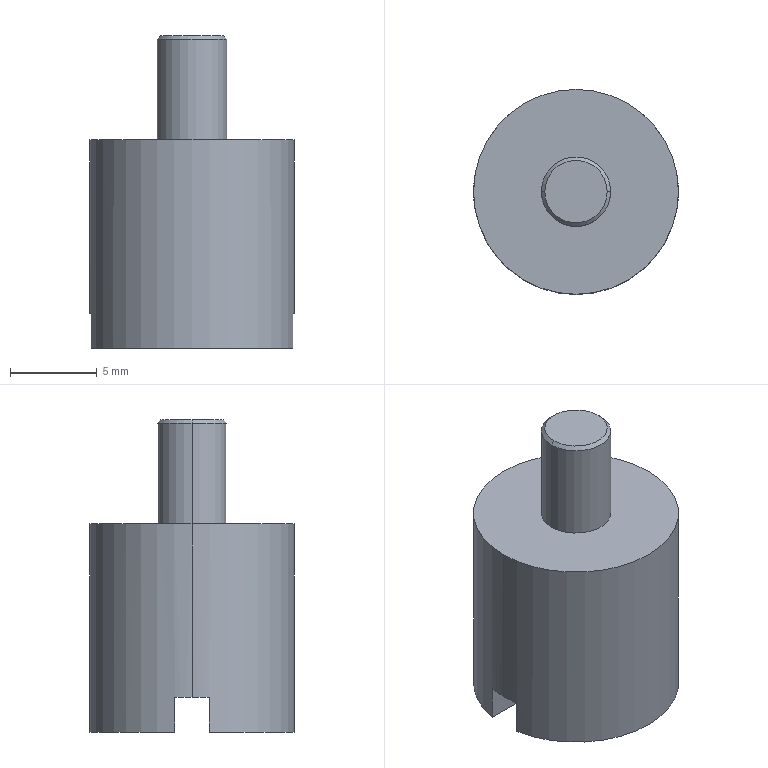Part | NX | features BREP 1 | 1 solid | 13 faces | box 11.8 x 11.8 x 18 mm | volume 1340 mm3 | plane 7 | cylinder 4 | cone 2 | commonest cylinder face diameters 4 x2 11.8 x2
STEP:
#1=CARTESIAN_POINT('',(-5.815,1.,2.));
#2=VERTEX_POINT('',#1);
#3=CARTESIAN_POINT('',(5.815,1.,2.));
#4=VERTEX_POINT('',#3);
#5=CARTESIAN_POINT('',(5.9,1.,2.));
#6=DIRECTION('',(1.,0.,0.));
#7=VECTOR('',#6,1000.);
#8=LINE('',#5,#7);
#9=EDGE_CURVE('',#2,#4,#8,.T.);
#10=ORIENTED_EDGE('',*,*,#9,.F.);
#11=CARTESIAN_POINT('',(-5.815,1.,0.));
#12=VERTEX_POINT('',#11);
#13=CARTESIAN_POINT('',(-5.815,1.,12.));
#14=DIRECTION('',(0.,0.,1.));
#15=VECTOR('',#14,1000.);
#16=LINE('',#13,#15);
#17=EDGE_CURVE('',#12,#2,#16,.T.);
#18=ORIENTED_EDGE('',*,*,#17,.F.);
#19=CARTESIAN_POINT('',(5.815,1.,0.));
#20=VERTEX_POINT('',#19);
#21=CARTESIAN_POINT('',(0.,1.,0.));
#22=DIRECTION('',(-1.,0.,0.));
#23=VECTOR('',#22,1000.);
#24=LINE('',#21,#23);
#25=EDGE_CURVE('',#20,#12,#24,.T.);
#26=ORIENTED_EDGE('',*,*,#25,.F.);
#27=CARTESIAN_POINT('',(5.815,1.,12.));
#28=DIRECTION('',(0.,0.,-1.));
#29=VECTOR('',#28,1000.);
#30=LINE('',#27,#29);
#31=EDGE_CURVE('',#4,#20,#30,.T.);
#32=ORIENTED_EDGE('',*,*,#31,.F.);
#33=EDGE_LOOP('',(#10,#18,#26,#32));
#34=FACE_BOUND('',#33,.T.);
#35=CARTESIAN_POINT('',(5.9,1.,2.));
#36=DIRECTION('',(0.,1.,0.));
#37=DIRECTION('',(0.,0.,1.));
#38=AXIS2_PLACEMENT_3D('',#35,#36,#37);
#39=PLANE('',#38);
#40=ADVANCED_FACE('',(#34),#39,.F.);
#41=CARTESIAN_POINT('',(5.815,-1.,2.));
#42=VERTEX_POINT('',#41);
#43=CARTESIAN_POINT('',(-5.815,-1.,2.));
#44=VERTEX_POINT('',#43);
#45=CARTESIAN_POINT('',(5.9,-1.,2.));
#46=DIRECTION('',(-1.,0.,0.));
#47=VECTOR('',#46,1000.);
#48=LINE('',#45,#47);
#49=EDGE_CURVE('',#42,#44,#48,.T.);
#50=ORIENTED_EDGE('',*,*,#49,.F.);
#51=CARTESIAN_POINT('',(5.815,-1.,0.));
#52=VERTEX_POINT('',#51);
#53=CARTESIAN_POINT('',(5.815,-1.,12.));
#54=DIRECTION('',(0.,0.,1.));
#55=VECTOR('',#54,1000.);
#56=LINE('',#53,#55);
#57=EDGE_CURVE('',#52,#42,#56,.T.);
#58=ORIENTED_EDGE('',*,*,#57,.F.);
#59=CARTESIAN_POINT('',(-5.815,-1.,0.));
#60=VERTEX_POINT('',#59);
#61=CARTESIAN_POINT('',(0.,-1.,0.));
#62=DIRECTION('',(1.,0.,0.));
#63=VECTOR('',#62,1000.);
#64=LINE('',#61,#63);
#65=EDGE_CURVE('',#60,#52,#64,.T.);
#66=ORIENTED_EDGE('',*,*,#65,.F.);
#67=CARTESIAN_POINT('',(-5.815,-1.,12.));
#68=DIRECTION('',(0.,0.,-1.));
#69=VECTOR('',#68,1000.);
#70=LINE('',#67,#69);
#71=EDGE_CURVE('',#44,#60,#70,.T.);
#72=ORIENTED_EDGE('',*,*,#71,.F.);
#73=EDGE_LOOP('',(#50,#58,#66,#72));
#74=FACE_BOUND('',#73,.T.);
#75=CARTESIAN_POINT('',(5.9,-1.,2.));
#76=DIRECTION('',(0.,-1.,0.));
#77=DIRECTION('',(0.,0.,-1.));
#78=AXIS2_PLACEMENT_3D('',#75,#76,#77);
#79=PLANE('',#78);
#80=ADVANCED_FACE('',(#74),#79,.F.);
#81=ORIENTED_EDGE('',*,*,#9,.T.);
#82=CARTESIAN_POINT('',(5.9,0.,2.));
#83=VERTEX_POINT('',#82);
#84=CARTESIAN_POINT('',(0.,0.,2.));
#85=DIRECTION('',(0.,0.,1.));
#86=DIRECTION('',(1.,0.,0.));
#87=AXIS2_PLACEMENT_3D('',#84,#85,#86);
#88=CIRCLE('',#87,5.9);
#89=EDGE_CURVE('',#83,#4,#88,.T.);
#90=ORIENTED_EDGE('',*,*,#89,.F.);
#91=CARTESIAN_POINT('',(0.,0.,2.));
#92=DIRECTION('',(0.,0.,1.));
#93=DIRECTION('',(1.,0.,0.));
#94=AXIS2_PLACEMENT_3D('',#91,#92,#93);
#95=CIRCLE('',#94,5.9);
#96=EDGE_CURVE('',#42,#83,#95,.T.);
#97=ORIENTED_EDGE('',*,*,#96,.F.);
#98=ORIENTED_EDGE('',*,*,#49,.T.);
#99=CARTESIAN_POINT('',(-5.9,0.,2.));
#100=VERTEX_POINT('',#99);
#101=CARTESIAN_POINT('',(0.,0.,2.));
#102=DIRECTION('',(0.,0.,1.));
#103=DIRECTION('',(1.,0.,0.));
#104=AXIS2_PLACEMENT_3D('',#101,#102,#103);
#105=CIRCLE('',#104,5.9);
#106=EDGE_CURVE('',#100,#44,#105,.T.);
#107=ORIENTED_EDGE('',*,*,#106,.F.);
#108=CARTESIAN_POINT('',(0.,0.,2.));
#109=DIRECTION('',(0.,0.,1.));
#110=DIRECTION('',(1.,0.,0.));
#111=AXIS2_PLACEMENT_3D('',#108,#109,#110);
#112=CIRCLE('',#111,5.9);
#113=EDGE_CURVE('',#2,#100,#112,.T.);
#114=ORIENTED_EDGE('',*,*,#113,.F.);
#115=EDGE_LOOP('',(#81,#90,#97,#98,#107,#114));
#116=FACE_BOUND('',#115,.T.);
#117=CARTESIAN_POINT('',(0.,0.,2.));
#118=DIRECTION('',(0.,0.,1.));
#119=DIRECTION('',(1.,0.,0.));
#120=AXIS2_PLACEMENT_3D('',#117,#118,#119);
#121=PLANE('',#120);
#122=ADVANCED_FACE('',(#116),#121,.F.);
#123=CARTESIAN_POINT('',(1.8,0.,18.));
#124=VERTEX_POINT('',#123);
#125=CARTESIAN_POINT('',(2.,0.,17.8));
#126=VERTEX_POINT('',#125);
#127=CARTESIAN_POINT('',(1.8,0.,18.));
#128=DIRECTION('',(0.7071,0.,-0.7071));
#129=VECTOR('',#128,1000.);
#130=LINE('',#127,#129);
#131=EDGE_CURVE('',#124,#126,#130,.T.);
#132=ORIENTED_EDGE('',*,*,#131,.F.);
#133=CARTESIAN_POINT('',(-1.8,0.,18.));
#134=VERTEX_POINT('',#133);
#135=CARTESIAN_POINT('',(0.,0.,18.));
#136=DIRECTION('',(0.,0.,1.));
#137=DIRECTION('',(1.,0.,0.));
#138=AXIS2_PLACEMENT_3D('',#135,#136,#137);
#139=CIRCLE('',#138,1.8);
#140=EDGE_CURVE('',#134,#124,#139,.T.);
#141=ORIENTED_EDGE('',*,*,#140,.F.);
#142=CARTESIAN_POINT('',(-2.,0.,17.8));
#143=VERTEX_POINT('',#142);
#144=CARTESIAN_POINT('',(-1.8,0.,18.));
#145=DIRECTION('',(-0.7071,0.,-0.7071));
#146=VECTOR('',#145,1000.);
#147=LINE('',#144,#146);
#148=EDGE_CURVE('',#134,#143,#147,.T.);
#149=ORIENTED_EDGE('',*,*,#148,.T.);
#150=CARTESIAN_POINT('',(0.,0.,17.8));
#151=DIRECTION('',(0.,0.,-1.));
#152=DIRECTION('',(1.,0.,0.));
#153=AXIS2_PLACEMENT_3D('',#150,#151,#152);
#154=CIRCLE('',#153,2.);
#155=EDGE_CURVE('',#126,#143,#154,.T.);
#156=ORIENTED_EDGE('',*,*,#155,.F.);
#157=EDGE_LOOP('',(#132,#141,#149,#156));
#158=FACE_BOUND('',#157,.T.);
#159=CARTESIAN_POINT('',(0.,0.,18.));
#160=DIRECTION('',(0.,0.,-1.));
#161=DIRECTION('',(-1.,0.,0.));
#162=AXIS2_PLACEMENT_3D('',#159,#160,#161);
#163=CONICAL_SURFACE('',#162,1.8,0.7854);
#164=ADVANCED_FACE('',(#158),#163,.T.);
#165=ORIENTED_EDGE('',*,*,#140,.T.);
#166=CARTESIAN_POINT('',(0.,0.,18.));
#167=DIRECTION('',(0.,0.,1.));
#168=DIRECTION('',(1.,0.,0.));
#169=AXIS2_PLACEMENT_3D('',#166,#167,#168);
#170=CIRCLE('',#169,1.8);
#171=EDGE_CURVE('',#124,#134,#170,.T.);
#172=ORIENTED_EDGE('',*,*,#171,.T.);
#173=EDGE_LOOP('',(#165,#172));
#174=FACE_BOUND('',#173,.T.);
#175=CARTESIAN_POINT('',(0.,0.,18.));
#176=DIRECTION('',(0.,0.,1.));
#177=DIRECTION('',(1.,0.,0.));
#178=AXIS2_PLACEMENT_3D('',#175,#176,#177);
#179=PLANE('',#178);
#180=ADVANCED_FACE('',(#174),#179,.T.);
#181=CARTESIAN_POINT('',(2.,0.,12.));
#182=VERTEX_POINT('',#181);
#183=CARTESIAN_POINT('',(2.,0.,18.));
#184=DIRECTION('',(0.,0.,-1.));
#185=VECTOR('',#184,1000.);
#186=LINE('',#183,#185);
#187=EDGE_CURVE('',#126,#182,#186,.T.);
#188=ORIENTED_EDGE('',*,*,#187,.F.);
#189=ORIENTED_EDGE('',*,*,#155,.T.);
#190=CARTESIAN_POINT('',(-2.,0.,12.));
#191=VERTEX_POINT('',#190);
#192=CARTESIAN_POINT('',(-2.,0.,18.));
#193=DIRECTION('',(0.,0.,-1.));
#194=VECTOR('',#193,1000.);
#195=LINE('',#192,#194);
#196=EDGE_CURVE('',#143,#191,#195,.T.);
#197=ORIENTED_EDGE('',*,*,#196,.T.);
#198=CARTESIAN_POINT('',(0.,0.,12.));
#199=DIRECTION('',(0.,0.,1.));
#200=DIRECTION('',(1.,0.,0.));
#201=AXIS2_PLACEMENT_3D('',#198,#199,#200);
#202=CIRCLE('',#201,2.);
#203=EDGE_CURVE('',#191,#182,#202,.T.);
#204=ORIENTED_EDGE('',*,*,#203,.T.);
#205=EDGE_LOOP('',(#188,#189,#197,#204));
#206=FACE_BOUND('',#205,.T.);
#207=CARTESIAN_POINT('',(0.,0.,18.));
#208=DIRECTION('',(0.,0.,-1.));
#209=DIRECTION('',(-1.,0.,0.));
#210=AXIS2_PLACEMENT_3D('',#207,#208,#209);
#211=CYLINDRICAL_SURFACE('',#210,2.);
#212=ADVANCED_FACE('',(#206),#211,.T.);
#213=CARTESIAN_POINT('',(0.,0.,0.));
#214=DIRECTION('',(0.,0.,1.));
#215=DIRECTION('',(1.,0.,0.));
#216=AXIS2_PLACEMENT_3D('',#213,#214,#215);
#217=CIRCLE('',#216,5.9);
#218=EDGE_CURVE('',#20,#12,#217,.T.);
#219=ORIENTED_EDGE('',*,*,#218,.F.);
#220=ORIENTED_EDGE('',*,*,#25,.T.);
#221=EDGE_LOOP('',(#219,#220));
#222=FACE_BOUND('',#221,.T.);
#223=CARTESIAN_POINT('',(0.,0.,0.));
#224=DIRECTION('',(0.,0.,1.));
#225=DIRECTION('',(1.,0.,0.));
#226=AXIS2_PLACEMENT_3D('',#223,#224,#225);
#227=PLANE('',#226);
#228=ADVANCED_FACE('',(#222),#227,.F.);
#229=CARTESIAN_POINT('',(-5.9,0.,12.));
#230=VERTEX_POINT('',#229);
#231=CARTESIAN_POINT('',(5.9,0.,12.));
#232=VERTEX_POINT('',#231);
#233=CARTESIAN_POINT('',(0.,0.,12.));
#234=DIRECTION('',(0.,0.,1.));
#235=DIRECTION('',(1.,0.,0.));
#236=AXIS2_PLACEMENT_3D('',#233,#234,#235);
#237=CIRCLE('',#236,5.9);
#238=EDGE_CURVE('',#230,#232,#237,.T.);
#239=ORIENTED_EDGE('',*,*,#238,.T.);
#240=CARTESIAN_POINT('',(0.,0.,12.));
#241=DIRECTION('',(0.,0.,1.));
#242=DIRECTION('',(1.,0.,0.));
#243=AXIS2_PLACEMENT_3D('',#240,#241,#242);
#244=CIRCLE('',#243,5.9);
#245=EDGE_CURVE('',#232,#230,#244,.T.);
#246=ORIENTED_EDGE('',*,*,#245,.T.);
#247=EDGE_LOOP('',(#239,#246));
#248=FACE_BOUND('',#247,.T.);
#249=ORIENTED_EDGE('',*,*,#203,.F.);
#250=CARTESIAN_POINT('',(0.,0.,12.));
#251=DIRECTION('',(0.,0.,1.));
#252=DIRECTION('',(1.,0.,0.));
#253=AXIS2_PLACEMENT_3D('',#250,#251,#252);
#254=CIRCLE('',#253,2.);
#255=EDGE_CURVE('',#182,#191,#254,.T.);
#256=ORIENTED_EDGE('',*,*,#255,.F.);
#257=EDGE_LOOP('',(#249,#256));
#258=FACE_BOUND('',#257,.T.);
#259=CARTESIAN_POINT('',(0.,0.,12.));
#260=DIRECTION('',(0.,0.,1.));
#261=DIRECTION('',(1.,0.,0.));
#262=AXIS2_PLACEMENT_3D('',#259,#260,#261);
#263=PLANE('',#262);
#264=ADVANCED_FACE('',(#248,#258),#263,.T.);
#265=CARTESIAN_POINT('',(5.9,0.,12.));
#266=DIRECTION('',(0.,0.,-1.));
#267=VECTOR('',#266,1000.);
#268=LINE('',#265,#267);
#269=EDGE_CURVE('',#232,#83,#268,.T.);
#270=ORIENTED_EDGE('',*,*,#269,.F.);
#271=ORIENTED_EDGE('',*,*,#238,.F.);
#272=CARTESIAN_POINT('',(-5.9,0.,12.));
#273=DIRECTION('',(0.,0.,-1.));
#274=VECTOR('',#273,1000.);
#275=LINE('',#272,#274);
#276=EDGE_CURVE('',#230,#100,#275,.T.);
#277=ORIENTED_EDGE('',*,*,#276,.T.);
#278=ORIENTED_EDGE('',*,*,#106,.T.);
#279=ORIENTED_EDGE('',*,*,#71,.T.);
#280=CARTESIAN_POINT('',(0.,0.,0.));
#281=DIRECTION('',(0.,0.,1.));
#282=DIRECTION('',(1.,0.,0.));
#283=AXIS2_PLACEMENT_3D('',#280,#281,#282);
#284=CIRCLE('',#283,5.9);
#285=EDGE_CURVE('',#60,#52,#284,.T.);
#286=ORIENTED_EDGE('',*,*,#285,.T.);
#287=ORIENTED_EDGE('',*,*,#57,.T.);
#288=ORIENTED_EDGE('',*,*,#96,.T.);
#289=EDGE_LOOP('',(#270,#271,#277,#278,#279,#286,#287,#288));
#290=FACE_BOUND('',#289,.T.);
#291=CARTESIAN_POINT('',(0.,0.,12.));
#292=DIRECTION('',(0.,0.,-1.));
#293=DIRECTION('',(-1.,0.,0.));
#294=AXIS2_PLACEMENT_3D('',#291,#292,#293);
#295=CYLINDRICAL_SURFACE('',#294,5.9);
#296=ADVANCED_FACE('',(#290),#295,.T.);
#297=ORIENTED_EDGE('',*,*,#285,.F.);
#298=ORIENTED_EDGE('',*,*,#65,.T.);
#299=EDGE_LOOP('',(#297,#298));
#300=FACE_BOUND('',#299,.T.);
#301=CARTESIAN_POINT('',(0.,0.,0.));
#302=DIRECTION('',(0.,0.,1.));
#303=DIRECTION('',(1.,0.,0.));
#304=AXIS2_PLACEMENT_3D('',#301,#302,#303);
#305=PLANE('',#304);
#306=ADVANCED_FACE('',(#300),#305,.F.);
#307=ORIENTED_EDGE('',*,*,#245,.F.);
#308=ORIENTED_EDGE('',*,*,#269,.T.);
#309=ORIENTED_EDGE('',*,*,#89,.T.);
#310=ORIENTED_EDGE('',*,*,#31,.T.);
#311=ORIENTED_EDGE('',*,*,#218,.T.);
#312=ORIENTED_EDGE('',*,*,#17,.T.);
#313=ORIENTED_EDGE('',*,*,#113,.T.);
#314=ORIENTED_EDGE('',*,*,#276,.F.);
#315=EDGE_LOOP('',(#307,#308,#309,#310,#311,#312,#313,#314));
#316=FACE_BOUND('',#315,.T.);
#317=CARTESIAN_POINT('',(0.,0.,12.));
#318=DIRECTION('',(0.,0.,-1.));
#319=DIRECTION('',(-1.,0.,0.));
#320=AXIS2_PLACEMENT_3D('',#317,#318,#319);
#321=CYLINDRICAL_SURFACE('',#320,5.9);
#322=ADVANCED_FACE('',(#316),#321,.T.);
#323=CARTESIAN_POINT('',(0.,0.,17.8));
#324=DIRECTION('',(0.,0.,-1.));
#325=DIRECTION('',(1.,0.,0.));
#326=AXIS2_PLACEMENT_3D('',#323,#324,#325);
#327=CIRCLE('',#326,2.);
#328=EDGE_CURVE('',#143,#126,#327,.T.);
#329=ORIENTED_EDGE('',*,*,#328,.T.);
#330=ORIENTED_EDGE('',*,*,#187,.T.);
#331=ORIENTED_EDGE('',*,*,#255,.T.);
#332=ORIENTED_EDGE('',*,*,#196,.F.);
#333=EDGE_LOOP('',(#329,#330,#331,#332));
#334=FACE_BOUND('',#333,.T.);
#335=CARTESIAN_POINT('',(0.,0.,18.));
#336=DIRECTION('',(0.,0.,-1.));
#337=DIRECTION('',(-1.,0.,0.));
#338=AXIS2_PLACEMENT_3D('',#335,#336,#337);
#339=CYLINDRICAL_SURFACE('',#338,2.);
#340=ADVANCED_FACE('',(#334),#339,.T.);
#341=ORIENTED_EDGE('',*,*,#171,.F.);
#342=ORIENTED_EDGE('',*,*,#131,.T.);
#343=ORIENTED_EDGE('',*,*,#328,.F.);
#344=ORIENTED_EDGE('',*,*,#148,.F.);
#345=EDGE_LOOP('',(#341,#342,#343,#344));
#346=FACE_BOUND('',#345,.T.);
#347=CARTESIAN_POINT('',(0.,0.,18.));
#348=DIRECTION('',(0.,0.,-1.));
#349=DIRECTION('',(-1.,0.,0.));
#350=AXIS2_PLACEMENT_3D('',#347,#348,#349);
#351=CONICAL_SURFACE('',#350,1.8,0.7854);
#352=ADVANCED_FACE('',(#346),#351,.T.);
#353=CLOSED_SHELL('',(#40,#80,#122,#164,#180,#212,#228,#264,#296,#306,#322,#340,#352));
#354=MANIFOLD_SOLID_BREP('',#353);
#355=(LENGTH_UNIT()NAMED_UNIT(*)SI_UNIT(.MILLI.,.METRE.));
#356=UNCERTAINTY_MEASURE_WITH_UNIT(LENGTH_MEASURE(0.00001),#355,'','');
#357=(NAMED_UNIT(*)PLANE_ANGLE_UNIT()SI_UNIT($,.RADIAN.));
#358=(NAMED_UNIT(*)SI_UNIT($,.STERADIAN.)SOLID_ANGLE_UNIT());
#359=(GEOMETRIC_REPRESENTATION_CONTEXT(3)GLOBAL_UNCERTAINTY_ASSIGNED_CONTEXT((#356))GLOBAL_UNIT_ASSIGNED_CONTEXT((#355,#357,#358))REPRESENTATION_CONTEXT('',''));
#360=ADVANCED_BREP_SHAPE_REPRESENTATION('',(#354),#359);